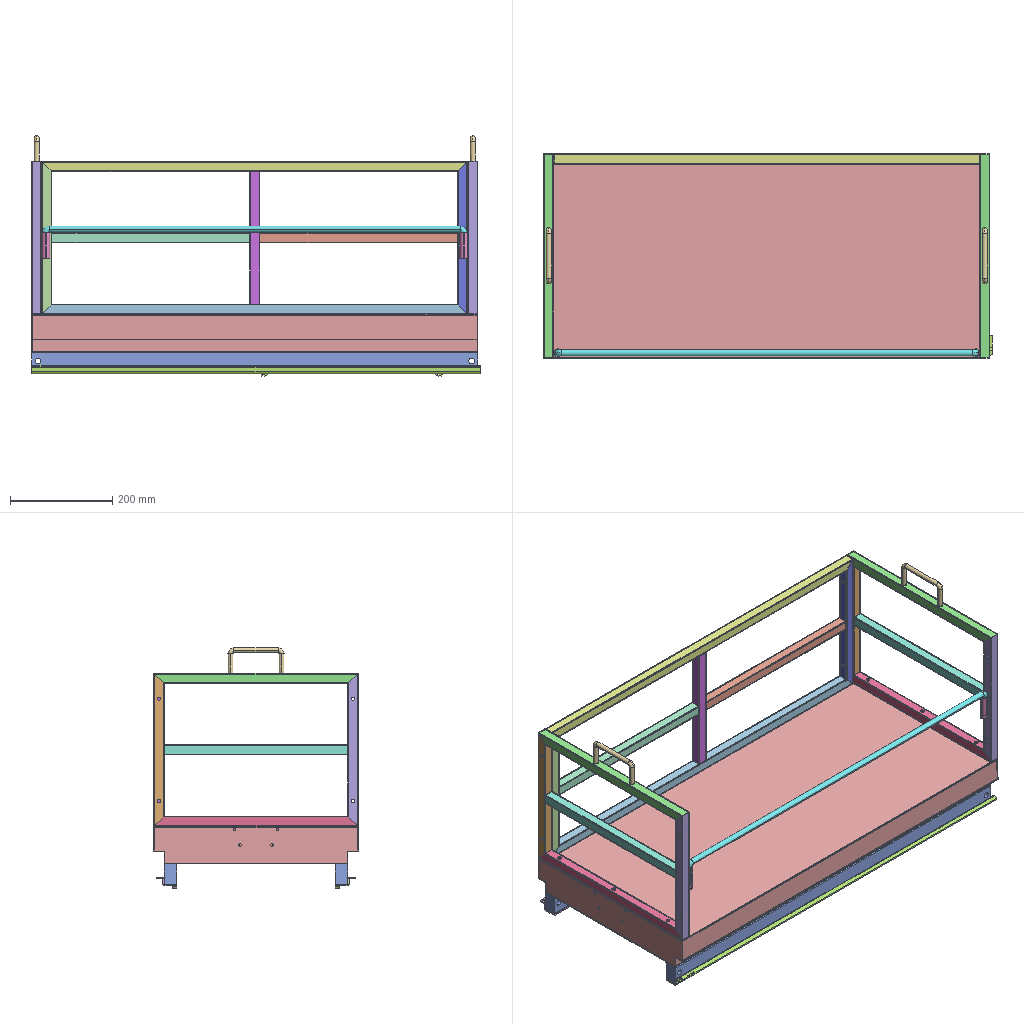Assembly | SolidWorks | 10 different items | 14 placed | box 880 x 400 x 471 mm
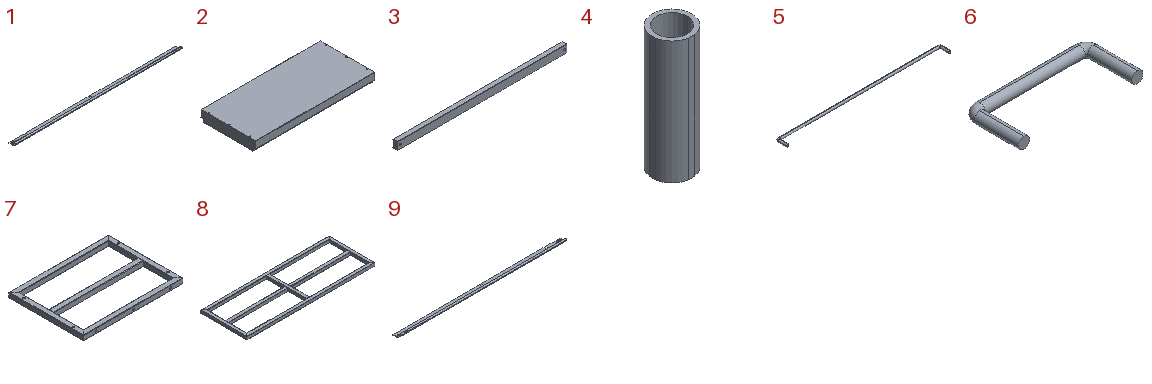Parts list (item | name | quantity | size | volume | features):
1 | - | x1 | 875 x 40 x 21.683 mm | 132017 mm3 | features ICE 3, EdgeFlange 2, FormToolInstance 2, SMBaseFlange 2, Fillet 1, FlatPattern 1, SheetMetal 1
2 | - | x1 | 875 x 400 x 73.5 mm | 926748 mm3 | features EdgeFlange 5, ICE 2, SMBaseFlange 2, CornerFeat 1, Cut 1, FlatPattern 1, SheetMetal 1
3 | - | x2 | 875 x 25 x 40 mm | 868078 mm3 | features Cut 1, Fillet 1, Sweep 1, WeldmentFeature 1
4 | - | x2 | 15.8 x 15.8 x 50 mm | 3884 mm3 | features Extrusion 1, ICE 1
5 | - | x1 | 831 x 56 x 12 mm | 103305 mm3 | features Sweep 1
6 | - | x2 | 110 x 50 x 10 mm | 14518 mm3 | features Sweep 1
7 | - | x2 | 400 x 300 x 20 mm | 147653 mm3 | features Cut 2, ICE 1, WeldMemberFeat 1, WeldmentFeature 1
8 | - | x1 | 835 x 300 x 20 mm | 284675 mm3 | features Cut 2, WeldMemberFeat 1, WeldmentFeature 1
9 | - | x1 | 880 x 40 x 21.683 mm | 132774 mm3 | features ICE 3, EdgeFlange 2, FormToolInstance 2, SMBaseFlange 2, Fillet 1, FlatPattern 1, SheetMetal 1
10 | Spring Support | x1 | - | - | -
Mates (type | each side: item.copy, entity, surface, feature):
Coincident | 2.1 face plane Edge-Flange4 | 3.1 face plane Sweep1
Coincident | 2.1 face plane Edge-Flange3 | 3.1 face plane Sweep1
Coincident | 2.1 face plane Edge-Flange1 | 3.1 face plane Sweep1
Coincident | 2.1 face plane Edge-Flange4 | 3.2 face plane Sweep1
Coincident | 2.1 face plane Edge-Flange3 | 3.2 face plane Sweep1
Coincident | 2.1 face plane Edge-Flange1 | 3.2 face plane Sweep1
Coincident | 3.2 face plane Sweep1 | 9.1 face plane Base-Flange1 | 2 times
Coincident | 3.2 face plane Sweep1 | 9.1 face plane Edge-Flange1
Coincident | 3.1 face plane Sweep1 | 1.1 face plane Base-Flange1 | 2 times
Coincident | 3.1 face plane Sweep1 | 1.1 face plane Edge-Flange1
Coincident | 2.1 face plane Base-Flange1 | 7.1 face plane Structural Member1
Coincident | 2.1 face plane Edge-Flange1 | 7.1 face plane Structural Member1 | 2 times
Coincident | 2.1 face plane Edge-Flange1 | 7.2 face plane Structural Member1 | 2 times
Coincident | 2.1 face plane Base-Flange1 | 7.2 face plane Structural Member1
Coincident | 7.1 face plane Structural Member1 | 8.1 face plane Structural Member1 | 2 times
Coincident | 2.1 face plane Base-Flange1 | 8.1 face plane Structural Member1
DistanceDim | 7.2 face plane Structural Member1 | 4.1 face plane Cut-Extrude1 | 2 times
Coincident | 7.2 face plane Structural Member1 | 4.1 face plane Boss-Extrude1
DistanceDim | 4.2 face plane Cut-Extrude1 | 7.1 face plane Structural Member1
Coincident | 4.1 face plane Cut-Extrude1 | 4.2 face plane Cut-Extrude1
Coincident | 7.1 face plane Structural Member1 | 4.2 face plane Boss-Extrude1
Concentric | 4.1 face cylinder Boss-Extrude1 | 5.1 face cylinder Sweep1
DistanceDim | 5.1 face plane Sweep1 | 4.1 face plane Boss-Extrude1
Tangent | 4.2 face cylinder Boss-Extrude1 | 5.1 face cylinder Sweep1
Coincident | 7.2 face plane Structural Member1 | 6.1 face plane Sweep1
Concentric | 7.2 face cylinder Cut-Extrude2 | 6.1 face cylinder Sweep1 | 2 times
Concentric | 7.1 face cylinder Cut-Extrude2 | 6.2 face cylinder Sweep1 | 2 times
Coincident | 7.1 face plane Structural Member1 | 6.2 face plane Sweep1